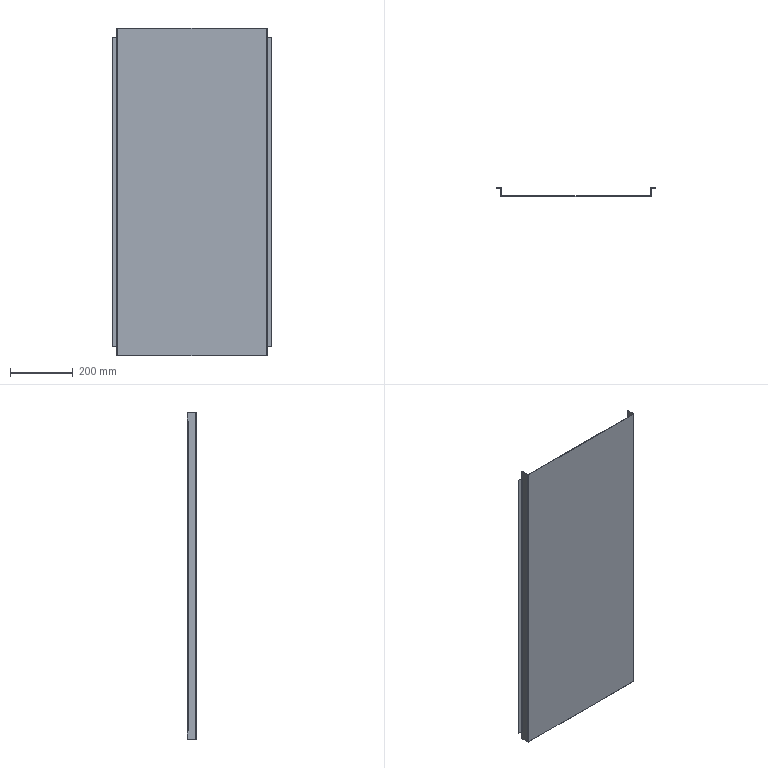Part | SolidWorks | features EdgeFlange 2, FlatPattern 1, SMBaseFlange 1, SheetMetal 1 | 1 solid | 46 faces | box 510 x 30 x 1047 mm | volume 882007 mm3 | plane 38 | cylinder 8 | commonest cylinder face diameters 3 x4 6 x4
STEP:
#1=CARTESIAN_POINT('',(-36.721,11.929,28.5));
#2=VERTEX_POINT('',#1);
#3=CARTESIAN_POINT('',(-36.721,11.527,28.5));
#4=VERTEX_POINT('',#3);
#5=CARTESIAN_POINT('',(-36.721,11.929,28.5));
#6=DIRECTION('',(0.,-1.,0.));
#7=VECTOR('',#6,1000.);
#8=LINE('',#5,#7);
#9=EDGE_CURVE('',#2,#4,#8,.T.);
#10=ORIENTED_EDGE('',*,*,#9,.T.);
#11=CARTESIAN_POINT('',(-35.221,8.929,28.5));
#12=VERTEX_POINT('',#11);
#13=CARTESIAN_POINT('',(-38.221,8.929,28.5));
#14=DIRECTION('',(0.,0.,-1.));
#15=DIRECTION('',(-1.,0.,0.));
#16=AXIS2_PLACEMENT_3D('',#13,#14,#15);
#17=CIRCLE('',#16,3.);
#18=EDGE_CURVE('',#4,#12,#17,.T.);
#19=ORIENTED_EDGE('',*,*,#18,.T.);
#20=CARTESIAN_POINT('',(-35.221,11.929,28.5));
#21=VERTEX_POINT('',#20);
#22=CARTESIAN_POINT('',(-35.221,0.,28.5));
#23=DIRECTION('',(0.,-1.,0.));
#24=VECTOR('',#23,1000.);
#25=LINE('',#22,#24);
#26=EDGE_CURVE('',#21,#12,#25,.T.);
#27=ORIENTED_EDGE('',*,*,#26,.F.);
#28=CARTESIAN_POINT('',(-36.721,11.929,28.5));
#29=DIRECTION('',(1.,0.,0.));
#30=VECTOR('',#29,1000.);
#31=LINE('',#28,#30);
#32=EDGE_CURVE('',#2,#21,#31,.T.);
#33=ORIENTED_EDGE('',*,*,#32,.F.);
#34=EDGE_LOOP('',(#10,#19,#27,#33));
#35=FACE_OUTER_BOUND('',#34,.T.);
#36=CARTESIAN_POINT('',(-36.721,11.929,28.5));
#37=DIRECTION('',(0.,0.,1.));
#38=DIRECTION('',(0.,-1.,0.));
#39=AXIS2_PLACEMENT_3D('',#36,#37,#38);
#40=PLANE('',#39);
#41=ADVANCED_FACE('',(#35),#40,.T.);
#42=CARTESIAN_POINT('',(-35.221,8.929,1018.5));
#43=VERTEX_POINT('',#42);
#44=CARTESIAN_POINT('',(-35.221,11.929,1018.5));
#45=VERTEX_POINT('',#44);
#46=CARTESIAN_POINT('',(-35.221,0.,1018.5));
#47=DIRECTION('',(0.,1.,0.));
#48=VECTOR('',#47,1000.);
#49=LINE('',#46,#48);
#50=EDGE_CURVE('',#43,#45,#49,.T.);
#51=ORIENTED_EDGE('',*,*,#50,.F.);
#52=CARTESIAN_POINT('',(-36.721,11.527,1018.5));
#53=VERTEX_POINT('',#52);
#54=CARTESIAN_POINT('',(-38.221,8.929,1018.5));
#55=DIRECTION('',(0.,0.,1.));
#56=DIRECTION('',(-1.,0.,0.));
#57=AXIS2_PLACEMENT_3D('',#54,#55,#56);
#58=CIRCLE('',#57,3.);
#59=EDGE_CURVE('',#43,#53,#58,.T.);
#60=ORIENTED_EDGE('',*,*,#59,.T.);
#61=CARTESIAN_POINT('',(-36.721,11.929,1018.5));
#62=VERTEX_POINT('',#61);
#63=CARTESIAN_POINT('',(-36.721,8.929,1018.5));
#64=DIRECTION('',(0.,1.,0.));
#65=VECTOR('',#64,1000.);
#66=LINE('',#63,#65);
#67=EDGE_CURVE('',#53,#62,#66,.T.);
#68=ORIENTED_EDGE('',*,*,#67,.T.);
#69=CARTESIAN_POINT('',(-36.721,11.929,1018.5));
#70=DIRECTION('',(1.,0.,0.));
#71=VECTOR('',#70,1000.);
#72=LINE('',#69,#71);
#73=EDGE_CURVE('',#62,#45,#72,.T.);
#74=ORIENTED_EDGE('',*,*,#73,.T.);
#75=EDGE_LOOP('',(#51,#60,#68,#74));
#76=FACE_OUTER_BOUND('',#75,.T.);
#77=CARTESIAN_POINT('',(-36.721,8.929,1018.5));
#78=DIRECTION('',(0.,0.,-1.));
#79=DIRECTION('',(-1.,0.,0.));
#80=AXIS2_PLACEMENT_3D('',#77,#78,#79);
#81=PLANE('',#80);
#82=ADVANCED_FACE('',(#76),#81,.T.);
#83=CARTESIAN_POINT('',(443.279,11.929,1018.5));
#84=VERTEX_POINT('',#83);
#85=CARTESIAN_POINT('',(443.279,11.527,1018.5));
#86=VERTEX_POINT('',#85);
#87=CARTESIAN_POINT('',(443.279,11.929,1018.5));
#88=DIRECTION('',(0.,-1.,0.));
#89=VECTOR('',#88,1000.);
#90=LINE('',#87,#89);
#91=EDGE_CURVE('',#84,#86,#90,.T.);
#92=ORIENTED_EDGE('',*,*,#91,.T.);
#93=CARTESIAN_POINT('',(441.779,8.929,1018.5));
#94=VERTEX_POINT('',#93);
#95=CARTESIAN_POINT('',(444.779,8.929,1018.5));
#96=DIRECTION('',(0.,0.,1.));
#97=DIRECTION('',(1.,0.,0.));
#98=AXIS2_PLACEMENT_3D('',#95,#96,#97);
#99=CIRCLE('',#98,3.);
#100=EDGE_CURVE('',#86,#94,#99,.T.);
#101=ORIENTED_EDGE('',*,*,#100,.T.);
#102=CARTESIAN_POINT('',(441.779,11.929,1018.5));
#103=VERTEX_POINT('',#102);
#104=CARTESIAN_POINT('',(441.779,0.,1018.5));
#105=DIRECTION('',(0.,1.,0.));
#106=VECTOR('',#105,1000.);
#107=LINE('',#104,#106);
#108=EDGE_CURVE('',#94,#103,#107,.T.);
#109=ORIENTED_EDGE('',*,*,#108,.T.);
#110=CARTESIAN_POINT('',(443.279,11.929,1018.5));
#111=DIRECTION('',(-1.,0.,0.));
#112=VECTOR('',#111,1000.);
#113=LINE('',#110,#112);
#114=EDGE_CURVE('',#84,#103,#113,.T.);
#115=ORIENTED_EDGE('',*,*,#114,.F.);
#116=EDGE_LOOP('',(#92,#101,#109,#115));
#117=FACE_OUTER_BOUND('',#116,.T.);
#118=CARTESIAN_POINT('',(443.279,11.929,1018.5));
#119=DIRECTION('',(0.,0.,-1.));
#120=DIRECTION('',(-1.,0.,0.));
#121=AXIS2_PLACEMENT_3D('',#118,#119,#120);
#122=PLANE('',#121);
#123=ADVANCED_FACE('',(#117),#122,.T.);
#124=CARTESIAN_POINT('',(441.779,11.929,28.5));
#125=VERTEX_POINT('',#124);
#126=CARTESIAN_POINT('',(441.779,8.929,28.5));
#127=VERTEX_POINT('',#126);
#128=CARTESIAN_POINT('',(441.779,0.,28.5));
#129=DIRECTION('',(0.,-1.,0.));
#130=VECTOR('',#129,1000.);
#131=LINE('',#128,#130);
#132=EDGE_CURVE('',#125,#127,#131,.T.);
#133=ORIENTED_EDGE('',*,*,#132,.T.);
#134=CARTESIAN_POINT('',(443.279,11.527,28.5));
#135=VERTEX_POINT('',#134);
#136=CARTESIAN_POINT('',(444.779,8.929,28.5));
#137=DIRECTION('',(0.,0.,-1.));
#138=DIRECTION('',(1.,0.,0.));
#139=AXIS2_PLACEMENT_3D('',#136,#137,#138);
#140=CIRCLE('',#139,3.);
#141=EDGE_CURVE('',#127,#135,#140,.T.);
#142=ORIENTED_EDGE('',*,*,#141,.T.);
#143=CARTESIAN_POINT('',(443.279,11.929,28.5));
#144=VERTEX_POINT('',#143);
#145=CARTESIAN_POINT('',(443.279,8.929,28.5));
#146=DIRECTION('',(0.,1.,0.));
#147=VECTOR('',#146,1000.);
#148=LINE('',#145,#147);
#149=EDGE_CURVE('',#135,#144,#148,.T.);
#150=ORIENTED_EDGE('',*,*,#149,.T.);
#151=CARTESIAN_POINT('',(443.279,11.929,28.5));
#152=DIRECTION('',(-1.,0.,0.));
#153=VECTOR('',#152,1000.);
#154=LINE('',#151,#153);
#155=EDGE_CURVE('',#144,#125,#154,.T.);
#156=ORIENTED_EDGE('',*,*,#155,.T.);
#157=EDGE_LOOP('',(#133,#142,#150,#156));
#158=FACE_OUTER_BOUND('',#157,.T.);
#159=CARTESIAN_POINT('',(443.279,8.929,28.5));
#160=DIRECTION('',(0.,0.,1.));
#161=DIRECTION('',(1.,0.,0.));
#162=AXIS2_PLACEMENT_3D('',#159,#160,#161);
#163=PLANE('',#162);
#164=ADVANCED_FACE('',(#158),#163,.T.);
#165=ORIENTED_EDGE('',*,*,#9,.F.);
#166=CARTESIAN_POINT('',(-36.721,11.929,0.));
#167=VERTEX_POINT('',#166);
#168=CARTESIAN_POINT('',(-36.721,11.929,0.));
#169=DIRECTION('',(0.,0.,1.));
#170=VECTOR('',#169,1000.);
#171=LINE('',#168,#170);
#172=EDGE_CURVE('',#167,#2,#171,.T.);
#173=ORIENTED_EDGE('',*,*,#172,.F.);
#174=CARTESIAN_POINT('',(-36.721,-15.071,0.));
#175=VERTEX_POINT('',#174);
#176=CARTESIAN_POINT('',(-36.721,-16.571,0.));
#177=DIRECTION('',(0.,1.,0.));
#178=VECTOR('',#177,1000.);
#179=LINE('',#176,#178);
#180=EDGE_CURVE('',#175,#167,#179,.T.);
#181=ORIENTED_EDGE('',*,*,#180,.F.);
#182=CARTESIAN_POINT('',(-36.721,-15.071,1047.));
#183=VERTEX_POINT('',#182);
#184=CARTESIAN_POINT('',(-36.721,-15.071,0.));
#185=DIRECTION('',(0.,0.,-1.));
#186=VECTOR('',#185,1000.);
#187=LINE('',#184,#186);
#188=EDGE_CURVE('',#183,#175,#187,.T.);
#189=ORIENTED_EDGE('',*,*,#188,.F.);
#190=CARTESIAN_POINT('',(-36.721,11.929,1047.));
#191=VERTEX_POINT('',#190);
#192=CARTESIAN_POINT('',(-36.721,11.929,1047.));
#193=DIRECTION('',(0.,-1.,0.));
#194=VECTOR('',#193,1000.);
#195=LINE('',#192,#194);
#196=EDGE_CURVE('',#191,#183,#195,.T.);
#197=ORIENTED_EDGE('',*,*,#196,.F.);
#198=CARTESIAN_POINT('',(-36.721,11.929,0.));
#199=DIRECTION('',(0.,0.,1.));
#200=VECTOR('',#199,1000.);
#201=LINE('',#198,#200);
#202=EDGE_CURVE('',#62,#191,#201,.T.);
#203=ORIENTED_EDGE('',*,*,#202,.F.);
#204=ORIENTED_EDGE('',*,*,#67,.F.);
#205=CARTESIAN_POINT('',(-36.721,8.929,1018.5));
#206=VERTEX_POINT('',#205);
#207=CARTESIAN_POINT('',(-36.721,8.929,1018.5));
#208=DIRECTION('',(0.,1.,0.));
#209=VECTOR('',#208,1000.);
#210=LINE('',#207,#209);
#211=EDGE_CURVE('',#206,#53,#210,.T.);
#212=ORIENTED_EDGE('',*,*,#211,.F.);
#213=CARTESIAN_POINT('',(-36.721,8.929,28.5));
#214=VERTEX_POINT('',#213);
#215=CARTESIAN_POINT('',(-36.721,8.929,28.5));
#216=DIRECTION('',(0.,0.,1.));
#217=VECTOR('',#216,1000.);
#218=LINE('',#215,#217);
#219=EDGE_CURVE('',#214,#206,#218,.T.);
#220=ORIENTED_EDGE('',*,*,#219,.F.);
#221=CARTESIAN_POINT('',(-36.721,11.929,28.5));
#222=DIRECTION('',(0.,-1.,0.));
#223=VECTOR('',#222,1000.);
#224=LINE('',#221,#223);
#225=EDGE_CURVE('',#4,#214,#224,.T.);
#226=ORIENTED_EDGE('',*,*,#225,.F.);
#227=EDGE_LOOP('',(#165,#173,#181,#189,#197,#203,#204,#212,#220,#226));
#228=FACE_OUTER_BOUND('',#227,.T.);
#229=CARTESIAN_POINT('',(-36.721,0.,0.));
#230=DIRECTION('',(1.,0.,0.));
#231=DIRECTION('',(0.,1.,0.));
#232=AXIS2_PLACEMENT_3D('',#229,#230,#231);
#233=PLANE('',#232);
#234=ADVANCED_FACE('',(#228),#233,.F.);
#235=CARTESIAN_POINT('',(-35.221,11.929,0.));
#236=VERTEX_POINT('',#235);
#237=CARTESIAN_POINT('',(-35.221,11.929,0.));
#238=DIRECTION('',(0.,0.,1.));
#239=VECTOR('',#238,1000.);
#240=LINE('',#237,#239);
#241=EDGE_CURVE('',#236,#21,#240,.T.);
#242=ORIENTED_EDGE('',*,*,#241,.T.);
#243=ORIENTED_EDGE('',*,*,#26,.T.);
#244=CARTESIAN_POINT('',(-35.221,8.929,28.5));
#245=DIRECTION('',(0.,0.,1.));
#246=VECTOR('',#245,1000.);
#247=LINE('',#244,#246);
#248=EDGE_CURVE('',#12,#43,#247,.T.);
#249=ORIENTED_EDGE('',*,*,#248,.T.);
#250=ORIENTED_EDGE('',*,*,#50,.T.);
#251=CARTESIAN_POINT('',(-35.221,11.929,1047.));
#252=VERTEX_POINT('',#251);
#253=CARTESIAN_POINT('',(-35.221,11.929,0.));
#254=DIRECTION('',(0.,0.,1.));
#255=VECTOR('',#254,1000.);
#256=LINE('',#253,#255);
#257=EDGE_CURVE('',#45,#252,#256,.T.);
#258=ORIENTED_EDGE('',*,*,#257,.T.);
#259=CARTESIAN_POINT('',(-35.221,-15.071,1047.));
#260=VERTEX_POINT('',#259);
#261=CARTESIAN_POINT('',(-35.221,0.,1047.));
#262=DIRECTION('',(0.,-1.,0.));
#263=VECTOR('',#262,1000.);
#264=LINE('',#261,#263);
#265=EDGE_CURVE('',#252,#260,#264,.T.);
#266=ORIENTED_EDGE('',*,*,#265,.T.);
#267=CARTESIAN_POINT('',(-35.221,-15.071,0.));
#268=VERTEX_POINT('',#267);
#269=CARTESIAN_POINT('',(-35.221,-15.071,0.));
#270=DIRECTION('',(0.,0.,1.));
#271=VECTOR('',#270,1000.);
#272=LINE('',#269,#271);
#273=EDGE_CURVE('',#268,#260,#272,.T.);
#274=ORIENTED_EDGE('',*,*,#273,.F.);
#275=CARTESIAN_POINT('',(-35.221,0.,0.));
#276=DIRECTION('',(0.,1.,0.));
#277=VECTOR('',#276,1000.);
#278=LINE('',#275,#277);
#279=EDGE_CURVE('',#268,#236,#278,.T.);
#280=ORIENTED_EDGE('',*,*,#279,.T.);
#281=EDGE_LOOP('',(#242,#243,#249,#250,#258,#266,#274,#280));
#282=FACE_OUTER_BOUND('',#281,.T.);
#283=CARTESIAN_POINT('',(-35.221,0.,0.));
#284=DIRECTION('',(1.,0.,0.));
#285=DIRECTION('',(0.,1.,0.));
#286=AXIS2_PLACEMENT_3D('',#283,#284,#285);
#287=PLANE('',#286);
#288=ADVANCED_FACE('',(#282),#287,.T.);
#289=ORIENTED_EDGE('',*,*,#172,.T.);
#290=ORIENTED_EDGE('',*,*,#32,.T.);
#291=ORIENTED_EDGE('',*,*,#241,.F.);
#292=CARTESIAN_POINT('',(-36.721,11.929,0.));
#293=DIRECTION('',(1.,0.,0.));
#294=VECTOR('',#293,1000.);
#295=LINE('',#292,#294);
#296=EDGE_CURVE('',#167,#236,#295,.T.);
#297=ORIENTED_EDGE('',*,*,#296,.F.);
#298=EDGE_LOOP('',(#289,#290,#291,#297));
#299=FACE_OUTER_BOUND('',#298,.T.);
#300=CARTESIAN_POINT('',(-36.721,11.929,0.));
#301=DIRECTION('',(0.,1.,0.));
#302=DIRECTION('',(-1.,0.,0.));
#303=AXIS2_PLACEMENT_3D('',#300,#301,#302);
#304=PLANE('',#303);
#305=ADVANCED_FACE('',(#299),#304,.T.);
#306=ORIENTED_EDGE('',*,*,#257,.F.);
#307=ORIENTED_EDGE('',*,*,#73,.F.);
#308=ORIENTED_EDGE('',*,*,#202,.T.);
#309=CARTESIAN_POINT('',(-36.721,11.929,1047.));
#310=DIRECTION('',(1.,0.,0.));
#311=VECTOR('',#310,1000.);
#312=LINE('',#309,#311);
#313=EDGE_CURVE('',#191,#252,#312,.T.);
#314=ORIENTED_EDGE('',*,*,#313,.T.);
#315=EDGE_LOOP('',(#306,#307,#308,#314));
#316=FACE_OUTER_BOUND('',#315,.T.);
#317=CARTESIAN_POINT('',(-36.721,11.929,0.));
#318=DIRECTION('',(0.,1.,0.));
#319=DIRECTION('',(-1.,0.,0.));
#320=AXIS2_PLACEMENT_3D('',#317,#318,#319);
#321=PLANE('',#320);
#322=ADVANCED_FACE('',(#316),#321,.T.);
#323=CARTESIAN_POINT('',(443.279,8.929,1018.5));
#324=VERTEX_POINT('',#323);
#325=CARTESIAN_POINT('',(443.279,8.929,28.5));
#326=VERTEX_POINT('',#325);
#327=CARTESIAN_POINT('',(443.279,8.929,1018.5));
#328=DIRECTION('',(0.,0.,-1.));
#329=VECTOR('',#328,1000.);
#330=LINE('',#327,#329);
#331=EDGE_CURVE('',#324,#326,#330,.T.);
#332=ORIENTED_EDGE('',*,*,#331,.F.);
#333=CARTESIAN_POINT('',(443.279,11.929,1018.5));
#334=DIRECTION('',(0.,-1.,0.));
#335=VECTOR('',#334,1000.);
#336=LINE('',#333,#335);
#337=EDGE_CURVE('',#86,#324,#336,.T.);
#338=ORIENTED_EDGE('',*,*,#337,.F.);
#339=ORIENTED_EDGE('',*,*,#91,.F.);
#340=CARTESIAN_POINT('',(443.279,11.929,1047.));
#341=VERTEX_POINT('',#340);
#342=CARTESIAN_POINT('',(443.279,11.929,0.));
#343=DIRECTION('',(0.,0.,-1.));
#344=VECTOR('',#343,1000.);
#345=LINE('',#342,#344);
#346=EDGE_CURVE('',#341,#84,#345,.T.);
#347=ORIENTED_EDGE('',*,*,#346,.F.);
#348=CARTESIAN_POINT('',(443.279,-15.071,1047.));
#349=VERTEX_POINT('',#348);
#350=CARTESIAN_POINT('',(443.279,11.929,1047.));
#351=DIRECTION('',(0.,1.,0.));
#352=VECTOR('',#351,1000.);
#353=LINE('',#350,#352);
#354=EDGE_CURVE('',#349,#341,#353,.T.);
#355=ORIENTED_EDGE('',*,*,#354,.F.);
#356=CARTESIAN_POINT('',(443.279,-15.071,0.));
#357=VERTEX_POINT('',#356);
#358=CARTESIAN_POINT('',(443.279,-15.071,0.));
#359=DIRECTION('',(0.,0.,-1.));
#360=VECTOR('',#359,1000.);
#361=LINE('',#358,#360);
#362=EDGE_CURVE('',#349,#357,#361,.T.);
#363=ORIENTED_EDGE('',*,*,#362,.T.);
#364=CARTESIAN_POINT('',(443.279,11.929,0.));
#365=VERTEX_POINT('',#364);
#366=CARTESIAN_POINT('',(443.279,-16.571,0.));
#367=DIRECTION('',(0.,-1.,0.));
#368=VECTOR('',#367,1000.);
#369=LINE('',#366,#368);
#370=EDGE_CURVE('',#365,#357,#369,.T.);
#371=ORIENTED_EDGE('',*,*,#370,.F.);
#372=CARTESIAN_POINT('',(443.279,11.929,0.));
#373=DIRECTION('',(0.,0.,-1.));
#374=VECTOR('',#373,1000.);
#375=LINE('',#372,#374);
#376=EDGE_CURVE('',#144,#365,#375,.T.);
#377=ORIENTED_EDGE('',*,*,#376,.F.);
#378=ORIENTED_EDGE('',*,*,#149,.F.);
#379=CARTESIAN_POINT('',(443.279,8.929,28.5));
#380=DIRECTION('',(0.,1.,0.));
#381=VECTOR('',#380,1000.);
#382=LINE('',#379,#381);
#383=EDGE_CURVE('',#326,#135,#382,.T.);
#384=ORIENTED_EDGE('',*,*,#383,.F.);
#385=EDGE_LOOP('',(#332,#338,#339,#347,#355,#363,#371,#377,#378,#384));
#386=FACE_OUTER_BOUND('',#385,.T.);
#387=CARTESIAN_POINT('',(443.279,0.,0.));
#388=DIRECTION('',(1.,0.,0.));
#389=DIRECTION('',(0.,1.,0.));
#390=AXIS2_PLACEMENT_3D('',#387,#388,#389);
#391=PLANE('',#390);
#392=ADVANCED_FACE('',(#386),#391,.T.);
#393=ORIENTED_EDGE('',*,*,#108,.F.);
#394=CARTESIAN_POINT('',(441.779,8.929,1018.5));
#395=DIRECTION('',(0.,0.,-1.));
#396=VECTOR('',#395,1000.);
#397=LINE('',#394,#396);
#398=EDGE_CURVE('',#94,#127,#397,.T.);
#399=ORIENTED_EDGE('',*,*,#398,.T.);
#400=ORIENTED_EDGE('',*,*,#132,.F.);
#401=CARTESIAN_POINT('',(441.779,11.929,0.));
#402=VERTEX_POINT('',#401);
#403=CARTESIAN_POINT('',(441.779,11.929,0.));
#404=DIRECTION('',(0.,0.,-1.));
#405=VECTOR('',#404,1000.);
#406=LINE('',#403,#405);
#407=EDGE_CURVE('',#125,#402,#406,.T.);
#408=ORIENTED_EDGE('',*,*,#407,.T.);
#409=CARTESIAN_POINT('',(441.779,-15.071,0.));
#410=VERTEX_POINT('',#409);
#411=CARTESIAN_POINT('',(441.779,0.,0.));
#412=DIRECTION('',(0.,-1.,0.));
#413=VECTOR('',#412,1000.);
#414=LINE('',#411,#413);
#415=EDGE_CURVE('',#402,#410,#414,.T.);
#416=ORIENTED_EDGE('',*,*,#415,.T.);
#417=CARTESIAN_POINT('',(441.779,-15.071,1047.));
#418=VERTEX_POINT('',#417);
#419=CARTESIAN_POINT('',(441.779,-15.071,1047.));
#420=DIRECTION('',(0.,0.,-1.));
#421=VECTOR('',#420,1000.);
#422=LINE('',#419,#421);
#423=EDGE_CURVE('',#418,#410,#422,.T.);
#424=ORIENTED_EDGE('',*,*,#423,.F.);
#425=CARTESIAN_POINT('',(441.779,11.929,1047.));
#426=VERTEX_POINT('',#425);
#427=CARTESIAN_POINT('',(441.779,0.,1047.));
#428=DIRECTION('',(0.,1.,0.));
#429=VECTOR('',#428,1000.);
#430=LINE('',#427,#429);
#431=EDGE_CURVE('',#418,#426,#430,.T.);
#432=ORIENTED_EDGE('',*,*,#431,.T.);
#433=CARTESIAN_POINT('',(441.779,11.929,0.));
#434=DIRECTION('',(0.,0.,-1.));
#435=VECTOR('',#434,1000.);
#436=LINE('',#433,#435);
#437=EDGE_CURVE('',#426,#103,#436,.T.);
#438=ORIENTED_EDGE('',*,*,#437,.T.);
#439=EDGE_LOOP('',(#393,#399,#400,#408,#416,#424,#432,#438));
#440=FACE_OUTER_BOUND('',#439,.T.);
#441=CARTESIAN_POINT('',(441.779,0.,0.));
#442=DIRECTION('',(1.,0.,0.));
#443=DIRECTION('',(0.,1.,0.));
#444=AXIS2_PLACEMENT_3D('',#441,#442,#443);
#445=PLANE('',#444);
#446=ADVANCED_FACE('',(#440),#445,.F.);
#447=ORIENTED_EDGE('',*,*,#346,.T.);
#448=ORIENTED_EDGE('',*,*,#114,.T.);
#449=ORIENTED_EDGE('',*,*,#437,.F.);
#450=CARTESIAN_POINT('',(443.279,11.929,1047.));
#451=DIRECTION('',(-1.,0.,0.));
#452=VECTOR('',#451,1000.);
#453=LINE('',#450,#452);
#454=EDGE_CURVE('',#341,#426,#453,.T.);
#455=ORIENTED_EDGE('',*,*,#454,.F.);
#456=EDGE_LOOP('',(#447,#448,#449,#455));
#457=FACE_OUTER_BOUND('',#456,.T.);
#458=CARTESIAN_POINT('',(443.279,11.929,0.));
#459=DIRECTION('',(0.,1.,0.));
#460=DIRECTION('',(-1.,0.,0.));
#461=AXIS2_PLACEMENT_3D('',#458,#459,#460);
#462=PLANE('',#461);
#463=ADVANCED_FACE('',(#457),#462,.T.);
#464=ORIENTED_EDGE('',*,*,#407,.F.);
#465=ORIENTED_EDGE('',*,*,#155,.F.);
#466=ORIENTED_EDGE('',*,*,#376,.T.);
#467=CARTESIAN_POINT('',(443.279,11.929,0.));
#468=DIRECTION('',(-1.,0.,0.));
#469=VECTOR('',#468,1000.);
#470=LINE('',#467,#469);
#471=EDGE_CURVE('',#365,#402,#470,.T.);
#472=ORIENTED_EDGE('',*,*,#471,.T.);
#473=EDGE_LOOP('',(#464,#465,#466,#472));
#474=FACE_OUTER_BOUND('',#473,.T.);
#475=CARTESIAN_POINT('',(443.279,11.929,0.));
#476=DIRECTION('',(0.,1.,0.));
#477=DIRECTION('',(-1.,0.,0.));
#478=AXIS2_PLACEMENT_3D('',#475,#476,#477);
#479=PLANE('',#478);
#480=ADVANCED_FACE('',(#474),#479,.T.);
#481=CARTESIAN_POINT('',(-33.721,-18.071,1047.));
#482=VERTEX_POINT('',#481);
#483=CARTESIAN_POINT('',(-33.721,-18.071,0.));
#484=VERTEX_POINT('',#483);
#485=CARTESIAN_POINT('',(-33.721,-18.071,1047.));
#486=DIRECTION('',(0.,0.,-1.));
#487=VECTOR('',#486,1000.);
#488=LINE('',#485,#487);
#489=EDGE_CURVE('',#482,#484,#488,.T.);
#490=ORIENTED_EDGE('',*,*,#489,.T.);
#491=CARTESIAN_POINT('',(440.279,-18.071,0.));
#492=VERTEX_POINT('',#491);
#493=CARTESIAN_POINT('',(-36.721,-18.071,0.));
#494=DIRECTION('',(1.,0.,0.));
#495=VECTOR('',#494,1000.);
#496=LINE('',#493,#495);
#497=EDGE_CURVE('',#484,#492,#496,.T.);
#498=ORIENTED_EDGE('',*,*,#497,.T.);
#499=CARTESIAN_POINT('',(440.279,-18.071,1047.));
#500=VERTEX_POINT('',#499);
#501=CARTESIAN_POINT('',(440.279,-18.071,0.));
#502=DIRECTION('',(0.,0.,1.));
#503=VECTOR('',#502,1000.);
#504=LINE('',#501,#503);
#505=EDGE_CURVE('',#492,#500,#504,.T.);
#506=ORIENTED_EDGE('',*,*,#505,.T.);
#507=CARTESIAN_POINT('',(-36.721,-18.071,1047.));
#508=DIRECTION('',(1.,0.,0.));
#509=VECTOR('',#508,1000.);
#510=LINE('',#507,#509);
#511=EDGE_CURVE('',#482,#500,#510,.T.);
#512=ORIENTED_EDGE('',*,*,#511,.F.);
#513=EDGE_LOOP('',(#490,#498,#506,#512));
#514=FACE_OUTER_BOUND('',#513,.T.);
#515=CARTESIAN_POINT('',(-36.721,-18.071,1047.));
#516=DIRECTION('',(0.,1.,0.));
#517=DIRECTION('',(0.,0.,1.));
#518=AXIS2_PLACEMENT_3D('',#515,#516,#517);
#519=PLANE('',#518);
#520=ADVANCED_FACE('',(#514),#519,.F.);
#521=CARTESIAN_POINT('',(-33.721,-16.571,0.));
#522=VERTEX_POINT('',#521);
#523=CARTESIAN_POINT('',(440.279,-16.571,0.));
#524=VERTEX_POINT('',#523);
#525=CARTESIAN_POINT('',(-36.721,-16.571,0.));
#526=DIRECTION('',(1.,0.,0.));
#527=VECTOR('',#526,1000.);
#528=LINE('',#525,#527);
#529=EDGE_CURVE('',#522,#524,#528,.T.);
#530=ORIENTED_EDGE('',*,*,#529,.F.);
#531=CARTESIAN_POINT('',(-33.721,-16.571,1047.));
#532=VERTEX_POINT('',#531);
#533=CARTESIAN_POINT('',(-33.721,-16.571,1047.));
#534=DIRECTION('',(0.,0.,-1.));
#535=VECTOR('',#534,1000.);
#536=LINE('',#533,#535);
#537=EDGE_CURVE('',#532,#522,#536,.T.);
#538=ORIENTED_EDGE('',*,*,#537,.F.);
#539=CARTESIAN_POINT('',(440.279,-16.571,1047.));
#540=VERTEX_POINT('',#539);
#541=CARTESIAN_POINT('',(-36.721,-16.571,1047.));
#542=DIRECTION('',(1.,0.,0.));
#543=VECTOR('',#542,1000.);
#544=LINE('',#541,#543);
#545=EDGE_CURVE('',#532,#540,#544,.T.);
#546=ORIENTED_EDGE('',*,*,#545,.T.);
#547=CARTESIAN_POINT('',(440.279,-16.571,0.));
#548=DIRECTION('',(0.,0.,1.));
#549=VECTOR('',#548,1000.);
#550=LINE('',#547,#549);
#551=EDGE_CURVE('',#524,#540,#550,.T.);
#552=ORIENTED_EDGE('',*,*,#551,.F.);
#553=EDGE_LOOP('',(#530,#538,#546,#552));
#554=FACE_OUTER_BOUND('',#553,.T.);
#555=CARTESIAN_POINT('',(-36.721,-16.571,1047.));
#556=DIRECTION('',(0.,1.,0.));
#557=DIRECTION('',(0.,0.,1.));
#558=AXIS2_PLACEMENT_3D('',#555,#556,#557);
#559=PLANE('',#558);
#560=ADVANCED_FACE('',(#554),#559,.T.);
#561=CARTESIAN_POINT('',(-33.721,-16.571,1047.));
#562=DIRECTION('',(0.,-1.,0.));
#563=VECTOR('',#562,1000.);
#564=LINE('',#561,#563);
#565=EDGE_CURVE('',#532,#482,#564,.T.);
#566=ORIENTED_EDGE('',*,*,#565,.T.);
#567=ORIENTED_EDGE('',*,*,#511,.T.);
#568=CARTESIAN_POINT('',(440.279,-16.571,1047.));
#569=DIRECTION('',(0.,-1.,0.));
#570=VECTOR('',#569,1000.);
#571=LINE('',#568,#570);
#572=EDGE_CURVE('',#540,#500,#571,.T.);
#573=ORIENTED_EDGE('',*,*,#572,.F.);
#574=ORIENTED_EDGE('',*,*,#545,.F.);
#575=EDGE_LOOP('',(#566,#567,#573,#574));
#576=FACE_OUTER_BOUND('',#575,.T.);
#577=CARTESIAN_POINT('',(0.,0.,1047.));
#578=DIRECTION('',(0.,0.,-1.));
#579=DIRECTION('',(-1.,0.,0.));
#580=AXIS2_PLACEMENT_3D('',#577,#578,#579);
#581=PLANE('',#580);
#582=ADVANCED_FACE('',(#576),#581,.F.);
#583=CARTESIAN_POINT('',(-33.721,-16.571,0.));
#584=DIRECTION('',(0.,-1.,0.));
#585=VECTOR('',#584,1000.);
#586=LINE('',#583,#585);
#587=EDGE_CURVE('',#522,#484,#586,.T.);
#588=ORIENTED_EDGE('',*,*,#587,.F.);
#589=ORIENTED_EDGE('',*,*,#529,.T.);
#590=CARTESIAN_POINT('',(440.279,-16.571,0.));
#591=DIRECTION('',(0.,-1.,0.));
#592=VECTOR('',#591,1000.);
#593=LINE('',#590,#592);
#594=EDGE_CURVE('',#524,#492,#593,.T.);
#595=ORIENTED_EDGE('',*,*,#594,.T.);
#596=ORIENTED_EDGE('',*,*,#497,.F.);
#597=EDGE_LOOP('',(#588,#589,#595,#596));
#598=FACE_OUTER_BOUND('',#597,.T.);
#599=CARTESIAN_POINT('',(0.,0.,0.));
#600=DIRECTION('',(0.,0.,-1.));
#601=DIRECTION('',(-1.,0.,0.));
#602=AXIS2_PLACEMENT_3D('',#599,#600,#601);
#603=PLANE('',#602);
#604=ADVANCED_FACE('',(#598),#603,.T.);
#605=CARTESIAN_POINT('',(443.279,-15.071,1047.));
#606=DIRECTION('',(1.,0.,0.));
#607=VECTOR('',#606,1000.);
#608=LINE('',#605,#607);
#609=EDGE_CURVE('',#418,#349,#608,.T.);
#610=ORIENTED_EDGE('',*,*,#609,.F.);
#611=CARTESIAN_POINT('',(440.279,-15.071,1047.));
#612=DIRECTION('',(0.,0.,1.));
#613=DIRECTION('',(0.,1.,0.));
#614=AXIS2_PLACEMENT_3D('',#611,#612,#613);
#615=CIRCLE('',#614,1.5);
#616=EDGE_CURVE('',#540,#418,#615,.T.);
#617=ORIENTED_EDGE('',*,*,#616,.F.);
#618=ORIENTED_EDGE('',*,*,#572,.T.);
#619=CARTESIAN_POINT('',(440.279,-15.071,1047.));
#620=DIRECTION('',(0.,0.,1.));
#621=DIRECTION('',(0.,1.,0.));
#622=AXIS2_PLACEMENT_3D('',#619,#620,#621);
#623=CIRCLE('',#622,3.);
#624=EDGE_CURVE('',#500,#349,#623,.T.);
#625=ORIENTED_EDGE('',*,*,#624,.T.);
#626=EDGE_LOOP('',(#610,#617,#618,#625));
#627=FACE_OUTER_BOUND('',#626,.T.);
#628=CARTESIAN_POINT('',(440.279,-15.071,1047.));
#629=DIRECTION('',(0.,0.,1.));
#630=DIRECTION('',(0.,-1.,0.));
#631=AXIS2_PLACEMENT_3D('',#628,#629,#630);
#632=PLANE('',#631);
#633=ADVANCED_FACE('',(#627),#632,.T.);
#634=CARTESIAN_POINT('',(440.279,-15.071,0.));
#635=DIRECTION('',(0.,0.,-1.));
#636=DIRECTION('',(0.,1.,0.));
#637=AXIS2_PLACEMENT_3D('',#634,#635,#636);
#638=CIRCLE('',#637,1.5);
#639=EDGE_CURVE('',#410,#524,#638,.T.);
#640=ORIENTED_EDGE('',*,*,#639,.F.);
#641=CARTESIAN_POINT('',(441.779,-15.071,0.));
#642=DIRECTION('',(1.,0.,0.));
#643=VECTOR('',#642,1000.);
#644=LINE('',#641,#643);
#645=EDGE_CURVE('',#410,#357,#644,.T.);
#646=ORIENTED_EDGE('',*,*,#645,.T.);
#647=CARTESIAN_POINT('',(440.279,-15.071,0.));
#648=DIRECTION('',(0.,0.,-1.));
#649=DIRECTION('',(0.,1.,0.));
#650=AXIS2_PLACEMENT_3D('',#647,#648,#649);
#651=CIRCLE('',#650,3.);
#652=EDGE_CURVE('',#357,#492,#651,.T.);
#653=ORIENTED_EDGE('',*,*,#652,.T.);
#654=ORIENTED_EDGE('',*,*,#594,.F.);
#655=EDGE_LOOP('',(#640,#646,#653,#654));
#656=FACE_OUTER_BOUND('',#655,.T.);
#657=CARTESIAN_POINT('',(440.279,-15.071,0.));
#658=DIRECTION('',(0.,0.,1.));
#659=DIRECTION('',(0.,-1.,0.));
#660=AXIS2_PLACEMENT_3D('',#657,#658,#659);
#661=PLANE('',#660);
#662=ADVANCED_FACE('',(#656),#661,.F.);
#663=ORIENTED_EDGE('',*,*,#505,.F.);
#664=ORIENTED_EDGE('',*,*,#652,.F.);
#665=ORIENTED_EDGE('',*,*,#362,.F.);
#666=ORIENTED_EDGE('',*,*,#624,.F.);
#667=EDGE_LOOP('',(#663,#664,#665,#666));
#668=FACE_OUTER_BOUND('',#667,.T.);
#669=CARTESIAN_POINT('',(440.279,-15.071,0.));
#670=DIRECTION('',(0.,0.,-1.));
#671=DIRECTION('',(1.,0.,0.));
#672=AXIS2_PLACEMENT_3D('',#669,#670,#671);
#673=CYLINDRICAL_SURFACE('',#672,3.);
#674=ADVANCED_FACE('',(#668),#673,.T.);
#675=ORIENTED_EDGE('',*,*,#551,.T.);
#676=ORIENTED_EDGE('',*,*,#616,.T.);
#677=ORIENTED_EDGE('',*,*,#423,.T.);
#678=ORIENTED_EDGE('',*,*,#639,.T.);
#679=EDGE_LOOP('',(#675,#676,#677,#678));
#680=FACE_OUTER_BOUND('',#679,.T.);
#681=CARTESIAN_POINT('',(440.279,-15.071,0.));
#682=DIRECTION('',(0.,0.,-1.));
#683=DIRECTION('',(1.,0.,0.));
#684=AXIS2_PLACEMENT_3D('',#681,#682,#683);
#685=CYLINDRICAL_SURFACE('',#684,1.5);
#686=ADVANCED_FACE('',(#680),#685,.F.);
#687=ORIENTED_EDGE('',*,*,#370,.T.);
#688=ORIENTED_EDGE('',*,*,#645,.F.);
#689=ORIENTED_EDGE('',*,*,#415,.F.);
#690=ORIENTED_EDGE('',*,*,#471,.F.);
#691=EDGE_LOOP('',(#687,#688,#689,#690));
#692=FACE_OUTER_BOUND('',#691,.T.);
#693=CARTESIAN_POINT('',(443.279,-16.571,0.));
#694=DIRECTION('',(0.,0.,-1.));
#695=DIRECTION('',(-1.,0.,0.));
#696=AXIS2_PLACEMENT_3D('',#693,#694,#695);
#697=PLANE('',#696);
#698=ADVANCED_FACE('',(#692),#697,.T.);
#699=ORIENTED_EDGE('',*,*,#431,.F.);
#700=ORIENTED_EDGE('',*,*,#609,.T.);
#701=ORIENTED_EDGE('',*,*,#354,.T.);
#702=ORIENTED_EDGE('',*,*,#454,.T.);
#703=EDGE_LOOP('',(#699,#700,#701,#702));
#704=FACE_OUTER_BOUND('',#703,.T.);
#705=CARTESIAN_POINT('',(443.279,11.929,1047.));
#706=DIRECTION('',(0.,0.,1.));
#707=DIRECTION('',(1.,0.,0.));
#708=AXIS2_PLACEMENT_3D('',#705,#706,#707);
#709=PLANE('',#708);
#710=ADVANCED_FACE('',(#704),#709,.T.);
#711=CARTESIAN_POINT('',(-36.721,-15.071,0.));
#712=DIRECTION('',(-1.,0.,0.));
#713=VECTOR('',#712,1000.);
#714=LINE('',#711,#713);
#715=EDGE_CURVE('',#268,#175,#714,.T.);
#716=ORIENTED_EDGE('',*,*,#715,.F.);
#717=CARTESIAN_POINT('',(-33.721,-15.071,0.));
#718=DIRECTION('',(0.,0.,-1.));
#719=DIRECTION('',(1.,0.,0.));
#720=AXIS2_PLACEMENT_3D('',#717,#718,#719);
#721=CIRCLE('',#720,1.5);
#722=EDGE_CURVE('',#522,#268,#721,.T.);
#723=ORIENTED_EDGE('',*,*,#722,.F.);
#724=ORIENTED_EDGE('',*,*,#587,.T.);
#725=CARTESIAN_POINT('',(-33.721,-15.071,0.));
#726=DIRECTION('',(0.,0.,-1.));
#727=DIRECTION('',(1.,0.,0.));
#728=AXIS2_PLACEMENT_3D('',#725,#726,#727);
#729=CIRCLE('',#728,3.);
#730=EDGE_CURVE('',#484,#175,#729,.T.);
#731=ORIENTED_EDGE('',*,*,#730,.T.);
#732=EDGE_LOOP('',(#716,#723,#724,#731));
#733=FACE_OUTER_BOUND('',#732,.T.);
#734=CARTESIAN_POINT('',(-33.721,-15.071,0.));
#735=DIRECTION('',(0.,0.,-1.));
#736=DIRECTION('',(-1.,0.,0.));
#737=AXIS2_PLACEMENT_3D('',#734,#735,#736);
#738=PLANE('',#737);
#739=ADVANCED_FACE('',(#733),#738,.T.);
#740=CARTESIAN_POINT('',(-33.721,-15.071,1047.));
#741=DIRECTION('',(0.,0.,1.));
#742=DIRECTION('',(1.,0.,0.));
#743=AXIS2_PLACEMENT_3D('',#740,#741,#742);
#744=CIRCLE('',#743,1.5);
#745=EDGE_CURVE('',#260,#532,#744,.T.);
#746=ORIENTED_EDGE('',*,*,#745,.F.);
#747=CARTESIAN_POINT('',(-35.221,-15.071,1047.));
#748=DIRECTION('',(-1.,0.,0.));
#749=VECTOR('',#748,1000.);
#750=LINE('',#747,#749);
#751=EDGE_CURVE('',#260,#183,#750,.T.);
#752=ORIENTED_EDGE('',*,*,#751,.T.);
#753=CARTESIAN_POINT('',(-33.721,-15.071,1047.));
#754=DIRECTION('',(0.,0.,1.));
#755=DIRECTION('',(1.,0.,0.));
#756=AXIS2_PLACEMENT_3D('',#753,#754,#755);
#757=CIRCLE('',#756,3.);
#758=EDGE_CURVE('',#183,#482,#757,.T.);
#759=ORIENTED_EDGE('',*,*,#758,.T.);
#760=ORIENTED_EDGE('',*,*,#565,.F.);
#761=EDGE_LOOP('',(#746,#752,#759,#760));
#762=FACE_OUTER_BOUND('',#761,.T.);
#763=CARTESIAN_POINT('',(-33.721,-15.071,1047.));
#764=DIRECTION('',(0.,0.,-1.));
#765=DIRECTION('',(-1.,0.,0.));
#766=AXIS2_PLACEMENT_3D('',#763,#764,#765);
#767=PLANE('',#766);
#768=ADVANCED_FACE('',(#762),#767,.F.);
#769=ORIENTED_EDGE('',*,*,#489,.F.);
#770=ORIENTED_EDGE('',*,*,#758,.F.);
#771=ORIENTED_EDGE('',*,*,#188,.T.);
#772=ORIENTED_EDGE('',*,*,#730,.F.);
#773=EDGE_LOOP('',(#769,#770,#771,#772));
#774=FACE_OUTER_BOUND('',#773,.T.);
#775=CARTESIAN_POINT('',(-33.721,-15.071,1047.));
#776=DIRECTION('',(0.,0.,1.));
#777=DIRECTION('',(-1.,0.,0.));
#778=AXIS2_PLACEMENT_3D('',#775,#776,#777);
#779=CYLINDRICAL_SURFACE('',#778,3.);
#780=ADVANCED_FACE('',(#774),#779,.T.);
#781=ORIENTED_EDGE('',*,*,#537,.T.);
#782=ORIENTED_EDGE('',*,*,#722,.T.);
#783=ORIENTED_EDGE('',*,*,#273,.T.);
#784=ORIENTED_EDGE('',*,*,#745,.T.);
#785=EDGE_LOOP('',(#781,#782,#783,#784));
#786=FACE_OUTER_BOUND('',#785,.T.);
#787=CARTESIAN_POINT('',(-33.721,-15.071,1047.));
#788=DIRECTION('',(0.,0.,1.));
#789=DIRECTION('',(-1.,0.,0.));
#790=AXIS2_PLACEMENT_3D('',#787,#788,#789);
#791=CYLINDRICAL_SURFACE('',#790,1.5);
#792=ADVANCED_FACE('',(#786),#791,.F.);
#793=ORIENTED_EDGE('',*,*,#279,.F.);
#794=ORIENTED_EDGE('',*,*,#715,.T.);
#795=ORIENTED_EDGE('',*,*,#180,.T.);
#796=ORIENTED_EDGE('',*,*,#296,.T.);
#797=EDGE_LOOP('',(#793,#794,#795,#796));
#798=FACE_OUTER_BOUND('',#797,.T.);
#799=CARTESIAN_POINT('',(-36.721,-16.571,0.));
#800=DIRECTION('',(0.,0.,-1.));
#801=DIRECTION('',(-1.,0.,0.));
#802=AXIS2_PLACEMENT_3D('',#799,#800,#801);
#803=PLANE('',#802);
#804=ADVANCED_FACE('',(#798),#803,.T.);
#805=ORIENTED_EDGE('',*,*,#196,.T.);
#806=ORIENTED_EDGE('',*,*,#751,.F.);
#807=ORIENTED_EDGE('',*,*,#265,.F.);
#808=ORIENTED_EDGE('',*,*,#313,.F.);
#809=EDGE_LOOP('',(#805,#806,#807,#808));
#810=FACE_OUTER_BOUND('',#809,.T.);
#811=CARTESIAN_POINT('',(-36.721,11.929,1047.));
#812=DIRECTION('',(0.,0.,1.));
#813=DIRECTION('',(1.,0.,0.));
#814=AXIS2_PLACEMENT_3D('',#811,#812,#813);
#815=PLANE('',#814);
#816=ADVANCED_FACE('',(#810),#815,.T.);
#817=CARTESIAN_POINT('',(444.779,10.429,28.5));
#818=VERTEX_POINT('',#817);
#819=CARTESIAN_POINT('',(444.779,8.929,28.5));
#820=DIRECTION('',(0.,0.,-1.));
#821=DIRECTION('',(1.,0.,0.));
#822=AXIS2_PLACEMENT_3D('',#819,#820,#821);
#823=CIRCLE('',#822,1.5);
#824=EDGE_CURVE('',#326,#818,#823,.T.);
#825=ORIENTED_EDGE('',*,*,#824,.F.);
#826=ORIENTED_EDGE('',*,*,#383,.T.);
#827=CARTESIAN_POINT('',(444.779,11.929,28.5));
#828=VERTEX_POINT('',#827);
#829=CARTESIAN_POINT('',(444.779,8.929,28.5));
#830=DIRECTION('',(0.,0.,-1.));
#831=DIRECTION('',(1.,0.,0.));
#832=AXIS2_PLACEMENT_3D('',#829,#830,#831);
#833=CIRCLE('',#832,3.);
#834=EDGE_CURVE('',#135,#828,#833,.T.);
#835=ORIENTED_EDGE('',*,*,#834,.T.);
#836=CARTESIAN_POINT('',(444.779,11.929,28.5));
#837=DIRECTION('',(0.,1.,0.));
#838=VECTOR('',#837,1000.);
#839=LINE('',#836,#838);
#840=EDGE_CURVE('',#818,#828,#839,.T.);
#841=ORIENTED_EDGE('',*,*,#840,.F.);
#842=EDGE_LOOP('',(#825,#826,#835,#841));
#843=FACE_OUTER_BOUND('',#842,.T.);
#844=CARTESIAN_POINT('',(444.779,8.929,28.5));
#845=DIRECTION('',(0.,0.,-1.));
#846=DIRECTION('',(-1.,0.,0.));
#847=AXIS2_PLACEMENT_3D('',#844,#845,#846);
#848=PLANE('',#847);
#849=ADVANCED_FACE('',(#843),#848,.T.);
#850=CARTESIAN_POINT('',(444.779,11.929,1018.5));
#851=VERTEX_POINT('',#850);
#852=CARTESIAN_POINT('',(444.779,8.929,1018.5));
#853=DIRECTION('',(0.,0.,1.));
#854=DIRECTION('',(1.,0.,0.));
#855=AXIS2_PLACEMENT_3D('',#852,#853,#854);
#856=CIRCLE('',#855,3.);
#857=EDGE_CURVE('',#851,#86,#856,.T.);
#858=ORIENTED_EDGE('',*,*,#857,.T.);
#859=ORIENTED_EDGE('',*,*,#337,.T.);
#860=CARTESIAN_POINT('',(444.779,10.429,1018.5));
#861=VERTEX_POINT('',#860);
#862=CARTESIAN_POINT('',(444.779,8.929,1018.5));
#863=DIRECTION('',(0.,0.,1.));
#864=DIRECTION('',(1.,0.,0.));
#865=AXIS2_PLACEMENT_3D('',#862,#863,#864);
#866=CIRCLE('',#865,1.5);
#867=EDGE_CURVE('',#861,#324,#866,.T.);
#868=ORIENTED_EDGE('',*,*,#867,.F.);
#869=CARTESIAN_POINT('',(444.779,10.429,1018.5));
#870=DIRECTION('',(0.,1.,0.));
#871=VECTOR('',#870,1000.);
#872=LINE('',#869,#871);
#873=EDGE_CURVE('',#861,#851,#872,.T.);
#874=ORIENTED_EDGE('',*,*,#873,.T.);
#875=EDGE_LOOP('',(#858,#859,#868,#874));
#876=FACE_OUTER_BOUND('',#875,.T.);
#877=CARTESIAN_POINT('',(444.779,8.929,1018.5));
#878=DIRECTION('',(0.,0.,-1.));
#879=DIRECTION('',(-1.,0.,0.));
#880=AXIS2_PLACEMENT_3D('',#877,#878,#879);
#881=PLANE('',#880);
#882=ADVANCED_FACE('',(#876),#881,.F.);
#883=ORIENTED_EDGE('',*,*,#398,.F.);
#884=ORIENTED_EDGE('',*,*,#100,.F.);
#885=ORIENTED_EDGE('',*,*,#857,.F.);
#886=CARTESIAN_POINT('',(444.779,11.929,28.5));
#887=DIRECTION('',(0.,0.,-1.));
#888=VECTOR('',#887,1000.);
#889=LINE('',#886,#888);
#890=EDGE_CURVE('',#851,#828,#889,.T.);
#891=ORIENTED_EDGE('',*,*,#890,.T.);
#892=ORIENTED_EDGE('',*,*,#834,.F.);
#893=ORIENTED_EDGE('',*,*,#141,.F.);
#894=EDGE_LOOP('',(#883,#884,#885,#891,#892,#893));
#895=FACE_OUTER_BOUND('',#894,.T.);
#896=CARTESIAN_POINT('',(444.779,8.929,1018.5));
#897=DIRECTION('',(0.,0.,1.));
#898=DIRECTION('',(0.,1.,0.));
#899=AXIS2_PLACEMENT_3D('',#896,#897,#898);
#900=CYLINDRICAL_SURFACE('',#899,3.);
#901=ADVANCED_FACE('',(#895),#900,.T.);
#902=ORIENTED_EDGE('',*,*,#331,.T.);
#903=ORIENTED_EDGE('',*,*,#824,.T.);
#904=CARTESIAN_POINT('',(444.779,10.429,28.5));
#905=DIRECTION('',(0.,0.,1.));
#906=VECTOR('',#905,1000.);
#907=LINE('',#904,#906);
#908=EDGE_CURVE('',#818,#861,#907,.T.);
#909=ORIENTED_EDGE('',*,*,#908,.T.);
#910=ORIENTED_EDGE('',*,*,#867,.T.);
#911=EDGE_LOOP('',(#902,#903,#909,#910));
#912=FACE_OUTER_BOUND('',#911,.T.);
#913=CARTESIAN_POINT('',(444.779,8.929,1018.5));
#914=DIRECTION('',(0.,0.,1.));
#915=DIRECTION('',(0.,1.,0.));
#916=AXIS2_PLACEMENT_3D('',#913,#914,#915);
#917=CYLINDRICAL_SURFACE('',#916,1.5);
#918=ADVANCED_FACE('',(#912),#917,.F.);
#919=ORIENTED_EDGE('',*,*,#873,.F.);
#920=CARTESIAN_POINT('',(458.279,10.429,1018.5));
#921=VERTEX_POINT('',#920);
#922=CARTESIAN_POINT('',(458.279,10.429,1018.5));
#923=DIRECTION('',(1.,0.,0.));
#924=VECTOR('',#923,1000.);
#925=LINE('',#922,#924);
#926=EDGE_CURVE('',#861,#921,#925,.T.);
#927=ORIENTED_EDGE('',*,*,#926,.T.);
#928=CARTESIAN_POINT('',(458.279,11.929,1018.5));
#929=VERTEX_POINT('',#928);
#930=CARTESIAN_POINT('',(458.279,11.929,1018.5));
#931=DIRECTION('',(0.,-1.,0.));
#932=VECTOR('',#931,1000.);
#933=LINE('',#930,#932);
#934=EDGE_CURVE('',#929,#921,#933,.T.);
#935=ORIENTED_EDGE('',*,*,#934,.F.);
#936=CARTESIAN_POINT('',(0.,11.929,1018.5));
#937=DIRECTION('',(1.,0.,0.));
#938=VECTOR('',#937,1000.);
#939=LINE('',#936,#938);
#940=EDGE_CURVE('',#851,#929,#939,.T.);
#941=ORIENTED_EDGE('',*,*,#940,.F.);
#942=EDGE_LOOP('',(#919,#927,#935,#941));
#943=FACE_OUTER_BOUND('',#942,.T.);
#944=CARTESIAN_POINT('',(458.279,11.929,1018.5));
#945=DIRECTION('',(0.,0.,-1.));
#946=DIRECTION('',(0.,1.,0.));
#947=AXIS2_PLACEMENT_3D('',#944,#945,#946);
#948=PLANE('',#947);
#949=ADVANCED_FACE('',(#943),#948,.F.);
#950=ORIENTED_EDGE('',*,*,#840,.T.);
#951=CARTESIAN_POINT('',(458.279,11.929,28.5));
#952=VERTEX_POINT('',#951);
#953=CARTESIAN_POINT('',(0.,11.929,28.5));
#954=DIRECTION('',(-1.,0.,0.));
#955=VECTOR('',#954,1000.);
#956=LINE('',#953,#955);
#957=EDGE_CURVE('',#952,#828,#956,.T.);
#958=ORIENTED_EDGE('',*,*,#957,.F.);
#959=CARTESIAN_POINT('',(458.279,10.429,28.5));
#960=VERTEX_POINT('',#959);
#961=CARTESIAN_POINT('',(458.279,11.929,28.5));
#962=DIRECTION('',(0.,-1.,0.));
#963=VECTOR('',#962,1000.);
#964=LINE('',#961,#963);
#965=EDGE_CURVE('',#952,#960,#964,.T.);
#966=ORIENTED_EDGE('',*,*,#965,.T.);
#967=CARTESIAN_POINT('',(443.279,10.429,28.5));
#968=DIRECTION('',(-1.,0.,0.));
#969=VECTOR('',#968,1000.);
#970=LINE('',#967,#969);
#971=EDGE_CURVE('',#960,#818,#970,.T.);
#972=ORIENTED_EDGE('',*,*,#971,.T.);
#973=EDGE_LOOP('',(#950,#958,#966,#972));
#974=FACE_OUTER_BOUND('',#973,.T.);
#975=CARTESIAN_POINT('',(443.279,11.929,28.5));
#976=DIRECTION('',(0.,0.,1.));
#977=DIRECTION('',(1.,0.,0.));
#978=AXIS2_PLACEMENT_3D('',#975,#976,#977);
#979=PLANE('',#978);
#980=ADVANCED_FACE('',(#974),#979,.F.);
#981=ORIENTED_EDGE('',*,*,#890,.F.);
#982=ORIENTED_EDGE('',*,*,#940,.T.);
#983=CARTESIAN_POINT('',(458.279,11.929,0.));
#984=DIRECTION('',(0.,0.,-1.));
#985=VECTOR('',#984,1000.);
#986=LINE('',#983,#985);
#987=EDGE_CURVE('',#929,#952,#986,.T.);
#988=ORIENTED_EDGE('',*,*,#987,.T.);
#989=ORIENTED_EDGE('',*,*,#957,.T.);
#990=EDGE_LOOP('',(#981,#982,#988,#989));
#991=FACE_OUTER_BOUND('',#990,.T.);
#992=CARTESIAN_POINT('',(0.,11.929,0.));
#993=DIRECTION('',(0.,-1.,0.));
#994=DIRECTION('',(1.,0.,0.));
#995=AXIS2_PLACEMENT_3D('',#992,#993,#994);
#996=PLANE('',#995);
#997=ADVANCED_FACE('',(#991),#996,.F.);
#998=ORIENTED_EDGE('',*,*,#926,.F.);
#999=ORIENTED_EDGE('',*,*,#908,.F.);
#1000=ORIENTED_EDGE('',*,*,#971,.F.);
#1001=CARTESIAN_POINT('',(458.279,10.429,28.5));
#1002=DIRECTION('',(0.,0.,-1.));
#1003=VECTOR('',#1002,1000.);
#1004=LINE('',#1001,#1003);
#1005=EDGE_CURVE('',#921,#960,#1004,.T.);
#1006=ORIENTED_EDGE('',*,*,#1005,.F.);
#1007=EDGE_LOOP('',(#998,#999,#1000,#1006));
#1008=FACE_OUTER_BOUND('',#1007,.T.);
#1009=CARTESIAN_POINT('',(0.,10.429,0.));
#1010=DIRECTION('',(0.,-1.,0.));
#1011=DIRECTION('',(1.,0.,0.));
#1012=AXIS2_PLACEMENT_3D('',#1009,#1010,#1011);
#1013=PLANE('',#1012);
#1014=ADVANCED_FACE('',(#1008),#1013,.T.);
#1015=ORIENTED_EDGE('',*,*,#1005,.T.);
#1016=ORIENTED_EDGE('',*,*,#965,.F.);
#1017=ORIENTED_EDGE('',*,*,#987,.F.);
#1018=ORIENTED_EDGE('',*,*,#934,.T.);
#1019=EDGE_LOOP('',(#1015,#1016,#1017,#1018));
#1020=FACE_OUTER_BOUND('',#1019,.T.);
#1021=CARTESIAN_POINT('',(458.279,11.929,28.5));
#1022=DIRECTION('',(-1.,0.,0.));
#1023=DIRECTION('',(0.,-1.,0.));
#1024=AXIS2_PLACEMENT_3D('',#1021,#1022,#1023);
#1025=PLANE('',#1024);
#1026=ADVANCED_FACE('',(#1020),#1025,.F.);
#1027=CARTESIAN_POINT('',(-38.221,10.429,1018.5));
#1028=VERTEX_POINT('',#1027);
#1029=CARTESIAN_POINT('',(-38.221,8.929,1018.5));
#1030=DIRECTION('',(0.,0.,1.));
#1031=DIRECTION('',(-1.,0.,0.));
#1032=AXIS2_PLACEMENT_3D('',#1029,#1030,#1031);
#1033=CIRCLE('',#1032,1.5);
#1034=EDGE_CURVE('',#206,#1028,#1033,.T.);
#1035=ORIENTED_EDGE('',*,*,#1034,.F.);
#1036=ORIENTED_EDGE('',*,*,#211,.T.);
#1037=CARTESIAN_POINT('',(-38.221,11.929,1018.5));
#1038=VERTEX_POINT('',#1037);
#1039=CARTESIAN_POINT('',(-38.221,8.929,1018.5));
#1040=DIRECTION('',(0.,0.,1.));
#1041=DIRECTION('',(-1.,0.,0.));
#1042=AXIS2_PLACEMENT_3D('',#1039,#1040,#1041);
#1043=CIRCLE('',#1042,3.);
#1044=EDGE_CURVE('',#53,#1038,#1043,.T.);
#1045=ORIENTED_EDGE('',*,*,#1044,.T.);
#1046=CARTESIAN_POINT('',(-38.221,11.929,1018.5));
#1047=DIRECTION('',(0.,1.,0.));
#1048=VECTOR('',#1047,1000.);
#1049=LINE('',#1046,#1048);
#1050=EDGE_CURVE('',#1028,#1038,#1049,.T.);
#1051=ORIENTED_EDGE('',*,*,#1050,.F.);
#1052=EDGE_LOOP('',(#1035,#1036,#1045,#1051));
#1053=FACE_OUTER_BOUND('',#1052,.T.);
#1054=CARTESIAN_POINT('',(-38.221,8.929,1018.5));
#1055=DIRECTION('',(0.,0.,1.));
#1056=DIRECTION('',(1.,0.,0.));
#1057=AXIS2_PLACEMENT_3D('',#1054,#1055,#1056);
#1058=PLANE('',#1057);
#1059=ADVANCED_FACE('',(#1053),#1058,.T.);
#1060=CARTESIAN_POINT('',(-38.221,11.929,28.5));
#1061=VERTEX_POINT('',#1060);
#1062=CARTESIAN_POINT('',(-38.221,8.929,28.5));
#1063=DIRECTION('',(0.,0.,-1.));
#1064=DIRECTION('',(-1.,0.,0.));
#1065=AXIS2_PLACEMENT_3D('',#1062,#1063,#1064);
#1066=CIRCLE('',#1065,3.);
#1067=EDGE_CURVE('',#1061,#4,#1066,.T.);
#1068=ORIENTED_EDGE('',*,*,#1067,.T.);
#1069=ORIENTED_EDGE('',*,*,#225,.T.);
#1070=CARTESIAN_POINT('',(-38.221,10.429,28.5));
#1071=VERTEX_POINT('',#1070);
#1072=CARTESIAN_POINT('',(-38.221,8.929,28.5));
#1073=DIRECTION('',(0.,0.,-1.));
#1074=DIRECTION('',(-1.,0.,0.));
#1075=AXIS2_PLACEMENT_3D('',#1072,#1073,#1074);
#1076=CIRCLE('',#1075,1.5);
#1077=EDGE_CURVE('',#1071,#214,#1076,.T.);
#1078=ORIENTED_EDGE('',*,*,#1077,.F.);
#1079=CARTESIAN_POINT('',(-38.221,10.429,28.5));
#1080=DIRECTION('',(0.,1.,0.));
#1081=VECTOR('',#1080,1000.);
#1082=LINE('',#1079,#1081);
#1083=EDGE_CURVE('',#1071,#1061,#1082,.T.);
#1084=ORIENTED_EDGE('',*,*,#1083,.T.);
#1085=EDGE_LOOP('',(#1068,#1069,#1078,#1084));
#1086=FACE_OUTER_BOUND('',#1085,.T.);
#1087=CARTESIAN_POINT('',(-38.221,8.929,28.5));
#1088=DIRECTION('',(0.,0.,1.));
#1089=DIRECTION('',(1.,0.,0.));
#1090=AXIS2_PLACEMENT_3D('',#1087,#1088,#1089);
#1091=PLANE('',#1090);
#1092=ADVANCED_FACE('',(#1086),#1091,.F.);
#1093=ORIENTED_EDGE('',*,*,#248,.F.);
#1094=ORIENTED_EDGE('',*,*,#18,.F.);
#1095=ORIENTED_EDGE('',*,*,#1067,.F.);
#1096=CARTESIAN_POINT('',(-38.221,11.929,1018.5));
#1097=DIRECTION('',(0.,0.,1.));
#1098=VECTOR('',#1097,1000.);
#1099=LINE('',#1096,#1098);
#1100=EDGE_CURVE('',#1061,#1038,#1099,.T.);
#1101=ORIENTED_EDGE('',*,*,#1100,.T.);
#1102=ORIENTED_EDGE('',*,*,#1044,.F.);
#1103=ORIENTED_EDGE('',*,*,#59,.F.);
#1104=EDGE_LOOP('',(#1093,#1094,#1095,#1101,#1102,#1103));
#1105=FACE_OUTER_BOUND('',#1104,.T.);
#1106=CARTESIAN_POINT('',(-38.221,8.929,28.5));
#1107=DIRECTION('',(0.,0.,-1.));
#1108=DIRECTION('',(0.,1.,0.));
#1109=AXIS2_PLACEMENT_3D('',#1106,#1107,#1108);
#1110=CYLINDRICAL_SURFACE('',#1109,3.);
#1111=ADVANCED_FACE('',(#1105),#1110,.T.);
#1112=ORIENTED_EDGE('',*,*,#219,.T.);
#1113=ORIENTED_EDGE('',*,*,#1034,.T.);
#1114=CARTESIAN_POINT('',(-38.221,10.429,1018.5));
#1115=DIRECTION('',(0.,0.,-1.));
#1116=VECTOR('',#1115,1000.);
#1117=LINE('',#1114,#1116);
#1118=EDGE_CURVE('',#1028,#1071,#1117,.T.);
#1119=ORIENTED_EDGE('',*,*,#1118,.T.);
#1120=ORIENTED_EDGE('',*,*,#1077,.T.);
#1121=EDGE_LOOP('',(#1112,#1113,#1119,#1120));
#1122=FACE_OUTER_BOUND('',#1121,.T.);
#1123=CARTESIAN_POINT('',(-38.221,8.929,28.5));
#1124=DIRECTION('',(0.,0.,-1.));
#1125=DIRECTION('',(0.,1.,0.));
#1126=AXIS2_PLACEMENT_3D('',#1123,#1124,#1125);
#1127=CYLINDRICAL_SURFACE('',#1126,1.5);
#1128=ADVANCED_FACE('',(#1122),#1127,.F.);
#1129=ORIENTED_EDGE('',*,*,#1083,.F.);
#1130=CARTESIAN_POINT('',(-51.721,10.429,28.5));
#1131=VERTEX_POINT('',#1130);
#1132=CARTESIAN_POINT('',(-51.721,10.429,28.5));
#1133=DIRECTION('',(-1.,0.,0.));
#1134=VECTOR('',#1133,1000.);
#1135=LINE('',#1132,#1134);
#1136=EDGE_CURVE('',#1071,#1131,#1135,.T.);
#1137=ORIENTED_EDGE('',*,*,#1136,.T.);
#1138=CARTESIAN_POINT('',(-51.721,11.929,28.5));
#1139=VERTEX_POINT('',#1138);
#1140=CARTESIAN_POINT('',(-51.721,11.929,28.5));
#1141=DIRECTION('',(0.,-1.,0.));
#1142=VECTOR('',#1141,1000.);
#1143=LINE('',#1140,#1142);
#1144=EDGE_CURVE('',#1139,#1131,#1143,.T.);
#1145=ORIENTED_EDGE('',*,*,#1144,.F.);
#1146=CARTESIAN_POINT('',(0.,11.929,28.5));
#1147=DIRECTION('',(-1.,0.,0.));
#1148=VECTOR('',#1147,1000.);
#1149=LINE('',#1146,#1148);
#1150=EDGE_CURVE('',#1061,#1139,#1149,.T.);
#1151=ORIENTED_EDGE('',*,*,#1150,.F.);
#1152=EDGE_LOOP('',(#1129,#1137,#1145,#1151));
#1153=FACE_OUTER_BOUND('',#1152,.T.);
#1154=CARTESIAN_POINT('',(-51.721,11.929,28.5));
#1155=DIRECTION('',(0.,0.,1.));
#1156=DIRECTION('',(1.,0.,0.));
#1157=AXIS2_PLACEMENT_3D('',#1154,#1155,#1156);
#1158=PLANE('',#1157);
#1159=ADVANCED_FACE('',(#1153),#1158,.F.);
#1160=ORIENTED_EDGE('',*,*,#1050,.T.);
#1161=CARTESIAN_POINT('',(-51.721,11.929,1018.5));
#1162=VERTEX_POINT('',#1161);
#1163=CARTESIAN_POINT('',(0.,11.929,1018.5));
#1164=DIRECTION('',(1.,0.,0.));
#1165=VECTOR('',#1164,1000.);
#1166=LINE('',#1163,#1165);
#1167=EDGE_CURVE('',#1162,#1038,#1166,.T.);
#1168=ORIENTED_EDGE('',*,*,#1167,.F.);
#1169=CARTESIAN_POINT('',(-51.721,10.429,1018.5));
#1170=VERTEX_POINT('',#1169);
#1171=CARTESIAN_POINT('',(-51.721,11.929,1018.5));
#1172=DIRECTION('',(0.,-1.,0.));
#1173=VECTOR('',#1172,1000.);
#1174=LINE('',#1171,#1173);
#1175=EDGE_CURVE('',#1162,#1170,#1174,.T.);
#1176=ORIENTED_EDGE('',*,*,#1175,.T.);
#1177=CARTESIAN_POINT('',(-36.721,10.429,1018.5));
#1178=DIRECTION('',(1.,0.,0.));
#1179=VECTOR('',#1178,1000.);
#1180=LINE('',#1177,#1179);
#1181=EDGE_CURVE('',#1170,#1028,#1180,.T.);
#1182=ORIENTED_EDGE('',*,*,#1181,.T.);
#1183=EDGE_LOOP('',(#1160,#1168,#1176,#1182));
#1184=FACE_OUTER_BOUND('',#1183,.T.);
#1185=CARTESIAN_POINT('',(-36.721,11.929,1018.5));
#1186=DIRECTION('',(0.,0.,-1.));
#1187=DIRECTION('',(0.,1.,0.));
#1188=AXIS2_PLACEMENT_3D('',#1185,#1186,#1187);
#1189=PLANE('',#1188);
#1190=ADVANCED_FACE('',(#1184),#1189,.F.);
#1191=ORIENTED_EDGE('',*,*,#1100,.F.);
#1192=ORIENTED_EDGE('',*,*,#1150,.T.);
#1193=CARTESIAN_POINT('',(-51.721,11.929,0.));
#1194=DIRECTION('',(0.,0.,1.));
#1195=VECTOR('',#1194,1000.);
#1196=LINE('',#1193,#1195);
#1197=EDGE_CURVE('',#1139,#1162,#1196,.T.);
#1198=ORIENTED_EDGE('',*,*,#1197,.T.);
#1199=ORIENTED_EDGE('',*,*,#1167,.T.);
#1200=EDGE_LOOP('',(#1191,#1192,#1198,#1199));
#1201=FACE_OUTER_BOUND('',#1200,.T.);
#1202=CARTESIAN_POINT('',(0.,11.929,0.));
#1203=DIRECTION('',(0.,-1.,0.));
#1204=DIRECTION('',(0.,0.,-1.));
#1205=AXIS2_PLACEMENT_3D('',#1202,#1203,#1204);
#1206=PLANE('',#1205);
#1207=ADVANCED_FACE('',(#1201),#1206,.F.);
#1208=ORIENTED_EDGE('',*,*,#1136,.F.);
#1209=ORIENTED_EDGE('',*,*,#1118,.F.);
#1210=ORIENTED_EDGE('',*,*,#1181,.F.);
#1211=CARTESIAN_POINT('',(-51.721,10.429,1018.5));
#1212=DIRECTION('',(0.,0.,1.));
#1213=VECTOR('',#1212,1000.);
#1214=LINE('',#1211,#1213);
#1215=EDGE_CURVE('',#1131,#1170,#1214,.T.);
#1216=ORIENTED_EDGE('',*,*,#1215,.F.);
#1217=EDGE_LOOP('',(#1208,#1209,#1210,#1216));
#1218=FACE_OUTER_BOUND('',#1217,.T.);
#1219=CARTESIAN_POINT('',(0.,10.429,0.));
#1220=DIRECTION('',(0.,-1.,0.));
#1221=DIRECTION('',(0.,0.,-1.));
#1222=AXIS2_PLACEMENT_3D('',#1219,#1220,#1221);
#1223=PLANE('',#1222);
#1224=ADVANCED_FACE('',(#1218),#1223,.T.);
#1225=ORIENTED_EDGE('',*,*,#1215,.T.);
#1226=ORIENTED_EDGE('',*,*,#1175,.F.);
#1227=ORIENTED_EDGE('',*,*,#1197,.F.);
#1228=ORIENTED_EDGE('',*,*,#1144,.T.);
#1229=EDGE_LOOP('',(#1225,#1226,#1227,#1228));
#1230=FACE_OUTER_BOUND('',#1229,.T.);
#1231=CARTESIAN_POINT('',(-51.721,11.929,1018.5));
#1232=DIRECTION('',(1.,0.,0.));
#1233=DIRECTION('',(0.,1.,0.));
#1234=AXIS2_PLACEMENT_3D('',#1231,#1232,#1233);
#1235=PLANE('',#1234);
#1236=ADVANCED_FACE('',(#1230),#1235,.F.);
#1237=CLOSED_SHELL('',(#41,#82,#123,#164,#234,#288,#305,#322,#392,#446,#463,#480,#520,#560,#582,#604,#633,#662,#674,#686,#698,#710,#739,#768,#780,#792,#804,#816,#849,#882,#901,#918,#949,#980,#997,#1014,#1026,#1059,#1092,#1111,#1128,#1159,#1190,#1207,#1224,#1236));
#1238=MANIFOLD_SOLID_BREP('',#1237);
#1239=CARTESIAN_POINT('',(0.,0.,0.));
#1240=DIRECTION('',(0.,0.,1.));
#1241=DIRECTION('',(1.,0.,0.));
#1242=AXIS2_PLACEMENT_3D('',#1239,#1240,#1241);
#1243=(LENGTH_UNIT()NAMED_UNIT(*)SI_UNIT(.MILLI.,.METRE.));
#1244=UNCERTAINTY_MEASURE_WITH_UNIT(LENGTH_MEASURE(0.00001),#1243,'','');
#1245=(NAMED_UNIT(*)PLANE_ANGLE_UNIT()SI_UNIT($,.RADIAN.));
#1246=(NAMED_UNIT(*)SI_UNIT($,.STERADIAN.)SOLID_ANGLE_UNIT());
#1247=(GEOMETRIC_REPRESENTATION_CONTEXT(3)GLOBAL_UNCERTAINTY_ASSIGNED_CONTEXT((#1244))GLOBAL_UNIT_ASSIGNED_CONTEXT((#1243,#1245,#1246))REPRESENTATION_CONTEXT('',''));
#1248=ADVANCED_BREP_SHAPE_REPRESENTATION('',(#1238,#1242),#1247);